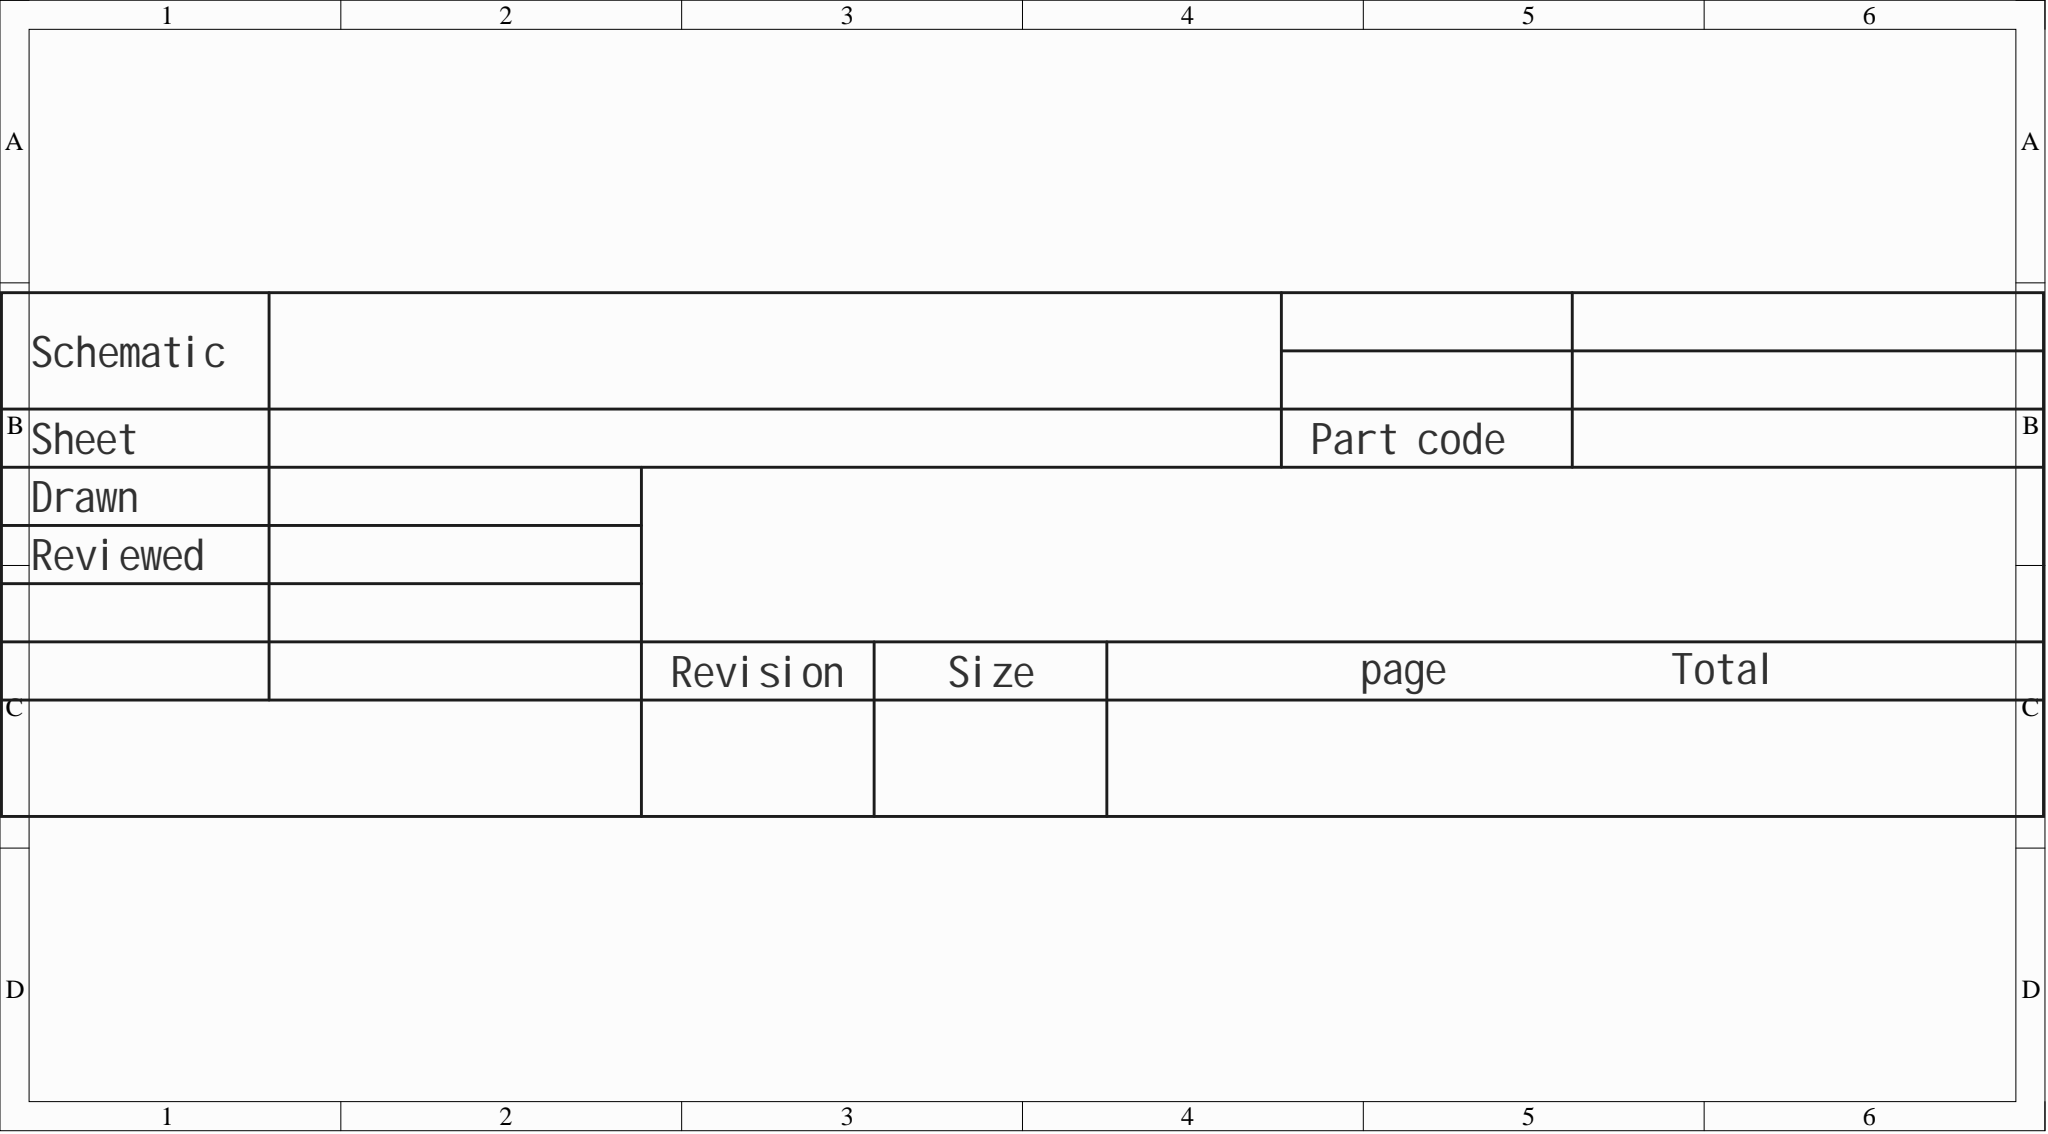Circuit board | Altium Designer | 26 parts | 46 nets
Bill of materials:
Comment,Description,Designator,Footprint,LibRef,Quantity
"buzzer","","BUZZER1","BUZ-TH_BD12.0-P6.00-D0.9-RD","buzzer","1"
"10uF","Capacitance:10uF; Tolerance:±20%; Rated voltage:250V; Ripple current:-; Equivalent series resistance:-;","C4","CAP-TH_BD6.3-P2.50-D1.0-FD","LKMC1202E100MF","1"
"22pF","","C7, C9","C0603","CAP_0603","2"
"100nF","","C8","C0805","CAP_0805","1"
"","","H1","HDR-TH_6P-P2.54-V-M-1","HDR-M_2.54_1x6P","1"
"","","H2","HDR-TH_4P-P2.54-V-F","HDR-F_2.54_1x4P","1"
"LMB162ADC","16x2 character LCD module","LCD1","LCD1602","LMB162ADC","1"
"","","Q1","S8550P_SOT","S8550_SOT_PNP","1"
"10kΩ","Resistance:10kΩ; Tolerance:±25%; Power:100mW;","R44","RES-ADJ-SMD_RM065-V1","RM065-103(10K)","1"
"10K","","R45, R47","R0603","Res_0603","2"
"1K","","R46, R51","R0603","Res_0603","2"
"100K","","R48, R49","R0603","Res_0603","2"
"50","","R50","R0603","Res_0603","1"
"MF52A502F3435","","R52","RES-TH_BD2.0-P1.80-D0.3","MF52A502F3435","1"
"2.2K","","R53","R0603","Res_0603","1"
"-","Number of resistors:-; Resistance:-; Power per element:-;","RN1","RES-ARRAY-TH_9P-P2.54-D1.0","排阻 10 K 5%","1"
"","","SW1, SW2","SW-TH_4P-L6.0-W6.0-P4.50-LS6.5","Key_TH_6x6x6","2"
"12MHz","Frequency:12MHz; Room-temperature frequency tolerance:±30ppm; External load capacitance:-; Frequency stability (full temperature):±50ppm;","U2","HC-49US_L11.0-W4.6-P4.88","ECS-120-S-4","1"
"STC89C516RD+40I-PDIP40","CPU core:51 series; Program storage capacity:61KB; Total RAM:1.25KB; GPIO port count:35; Operating voltage range:3.5V~5.5V; CPU max clock:-; Program memory type:FLASH;","U3","DIP-40_L52.3-W13.9-P2.54-LS15.2-BL","STC89C516RD+40I-PDIP40","1"
"AD1674AD","Interface:Parallel; Supply voltage:11.4V~16.5V; Sampling rate:100kHz; Resolution:12 bit;","U5","CDIP-28_L35.5-W14.8-P2.54-LS15.3-BL","AD1674AD","1"
"LM358P-CN","","U7","SOIC-8_L5.0-W4.0-P1.27-LS6.0-BL","LM358P-CN","1"
Netlist (Protel format):
[
BUZZER1
BUZ-TH_BD12.0-P6.00-D0.9-RD
buzzer



]
[
C4
CAP-TH_BD6.3-P2.50-D1.0-FD
10uF



]
[
C7
C0603
22pF



]
[
C8
C0805
100nF



]
[
C9
C0603
22pF



]
[
H1
HDR-TH_6P-P2.54-V-M-1




]
[
H2
HDR-TH_4P-P2.54-V-F




]
[
LCD1
LCD1602
LMB162ADC



]
[
Q1
S8550P_SOT




]
[
R44
RES-ADJ-SMD_RM065-V1
10kΩ



]
[
R45
R0603
10K



]
[
R46
R0603
1K



]
[
R47
R0603
10K



]
[
R48
R0603
100K



]
[
R49
R0603
100K



]
[
R50
R0603
50



]
[
R51
R0603
1K



]
[
R52
RES-TH_BD2.0-P1.80-D0.3
MF52A502F3435



]
[
R53
R0603
2.2K



]
[
RN1
RES-ARRAY-TH_9P-P2.54-D1.0
-



]
[
SW1
SW-TH_4P-L6.0-W6.0-P4.50-LS6.5




]
[
SW2
SW-TH_4P-L6.0-W6.0-P4.50-LS6.5




]
[
U2
HC-49US_L11.0-W4.6-P4.88
12MHz



]
[
U3
DIP-40_L52.3-W13.9-P2.54-LS15.2-BL
STC89C516RD+40I-PDIP40



]
[
U5
CDIP-28_L35.5-W14.8-P2.54-LS15.3-BL
AD1674AD



]
[
U7
SOIC-8_L5.0-W4.0-P1.27-LS6.0-BL
LM358P-CN



]
(
VCC
C4-1
H1-1
H2-1
LCD1-2
LCD1-15
Q1-2
R45-2
RN1-1
U3-40
)
(
RW
LCD1-5
U3-27
)
(
RS
LCD1-4
U3-26
)
(
RC
U3-25
U5-5
)
(
NetU3_8
U3-8
U5-19
U5-27
)
(
NetU3_7
U3-7
U5-18
U5-26
)
(
NetU3_6
U3-6
U5-17
U5-25
)
(
NetU3_5
U3-5
U5-16
U5-24
)
(
NetU3_4
U3-4
U5-23
)
(
NetU3_3
U3-3
U5-22
)
(
NetU3_2
U3-2
U5-21
)
(
NetU3_1
U3-1
U5-20
)
(
NetSW2_3
SW2-3
U3-13
)
(
NetSW1_3
SW1-3
U3-12
)
(
NetR53_1
R53-1
U3-17
)
(
NetR51_1
R51-1
R52-2
U7-3
)
(
NetR50_2
R50-2
U5-8
)
(
NetR50_1
R50-1
U5-10
)
(
NetR48_1
R48-1
R49-1
U5-12
)
(
NetR44_2
R44-2
R49-2
)
(
NetQ1_1
Q1-1
R53-2
)
(
NetLCD1_14
LCD1-14
RN1-9
U3-32
)
(
NetLCD1_13
LCD1-13
RN1-8
U3-33
)
(
NetLCD1_12
LCD1-12
RN1-7
U3-34
)
(
NetLCD1_11
LCD1-11
RN1-6
U3-35
)
(
NetLCD1_10
LCD1-10
RN1-5
U3-36
)
(
NetLCD1_9
LCD1-9
RN1-4
U3-37
)
(
NetLCD1_8
LCD1-8
RN1-3
U3-38
)
(
NetLCD1_7
LCD1-7
RN1-2
U3-39
)
(
NetLCD1_3
LCD1-3
R45-1
R46-2
)
(
NetH2_4
H2-4
U3-11
)
(
NetH2_3
H2-3
U3-10
)
(
NetC9_2
C9-2
U2-2
U3-19
)
(
NetC8_2
C8-2
U5-13
U7-1
U7-2
U7-8
)
(
NetC7_2
C7-2
U2-1
U3-18
)
(
NetC4_2
C4-2
R47-2
U3-9
)
(
NetBUZZER1_2
BUZZER1-2
Q1-3
)
(
GND
BUZZER1-1
C7-1
C8-1
C9-1
H1-6
H2-2
LCD1-1
LCD1-16
R46-1
R47-1
R48-2
R52-1
SW1-1
SW1-2
SW2-1
SW2-2
U3-20
U5-2
)
(
EN
LCD1-6
U3-28
)
(
CS
U3-22
U5-3
)
(
CE
U3-24
U5-6
)
(
AD
U3-23
U5-4
)
(
-15V
H1-5
U5-11
)
(
+16V
H1-3
U5-7
)
(
+12V
H1-4
R44-1
)
(
+6V
H1-2
R51-2
U7-4
)